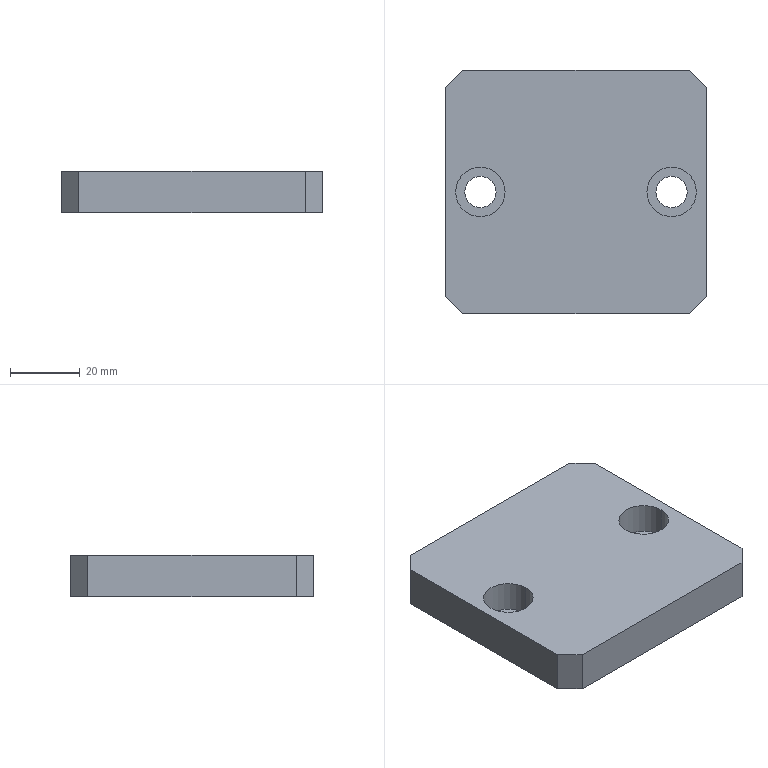Part | Creo | 1 solid | 20 faces | box 75 x 70 x 12 mm | volume 59148 mm3 | plane 12 | cylinder 8 | commonest cylinder face diameters 9 x4 14.25 x4
STEP:
#1=CARTESIAN_POINT('',(0.,0.,0.));
#2=DIRECTION('',(0.,0.,1.));
#3=DIRECTION('',(1.,0.,0.));
#4=AXIS2_PLACEMENT_3D('',#1,#2,#3);
#5=CARTESIAN_POINT('',(311.601,202.373,-28.441));
#6=VERTEX_POINT('',#5);
#7=CARTESIAN_POINT('',(311.601,262.373,-28.441));
#8=VERTEX_POINT('',#7);
#9=CARTESIAN_POINT('',(311.601,202.373,-28.441));
#10=DIRECTION('',(0.,1.,0.));
#11=VECTOR('',#10,60.);
#12=LINE('',#9,#11);
#13=EDGE_CURVE('',#6,#8,#12,.T.);
#14=ORIENTED_EDGE('',*,*,#13,.T.);
#15=CARTESIAN_POINT('',(316.601,267.373,-28.441));
#16=VERTEX_POINT('',#15);
#17=CARTESIAN_POINT('',(316.601,267.373,-28.441));
#18=DIRECTION('',(-0.7071,-0.7071,0.));
#19=VECTOR('',#18,7.071);
#20=LINE('',#17,#19);
#21=EDGE_CURVE('',#16,#8,#20,.T.);
#22=ORIENTED_EDGE('',*,*,#21,.F.);
#23=CARTESIAN_POINT('',(381.601,267.373,-28.441));
#24=VERTEX_POINT('',#23);
#25=CARTESIAN_POINT('',(316.601,267.373,-28.441));
#26=DIRECTION('',(1.,0.,0.));
#27=VECTOR('',#26,65.);
#28=LINE('',#25,#27);
#29=EDGE_CURVE('',#16,#24,#28,.T.);
#30=ORIENTED_EDGE('',*,*,#29,.T.);
#31=CARTESIAN_POINT('',(386.601,262.373,-28.441));
#32=VERTEX_POINT('',#31);
#33=CARTESIAN_POINT('',(386.601,262.373,-28.441));
#34=DIRECTION('',(-0.7071,0.7071,0.));
#35=VECTOR('',#34,7.071);
#36=LINE('',#33,#35);
#37=EDGE_CURVE('',#32,#24,#36,.T.);
#38=ORIENTED_EDGE('',*,*,#37,.F.);
#39=CARTESIAN_POINT('',(386.601,202.373,-28.441));
#40=VERTEX_POINT('',#39);
#41=CARTESIAN_POINT('',(386.601,262.373,-28.441));
#42=DIRECTION('',(0.,-1.,0.));
#43=VECTOR('',#42,60.);
#44=LINE('',#41,#43);
#45=EDGE_CURVE('',#32,#40,#44,.T.);
#46=ORIENTED_EDGE('',*,*,#45,.T.);
#47=CARTESIAN_POINT('',(381.601,197.373,-28.441));
#48=VERTEX_POINT('',#47);
#49=CARTESIAN_POINT('',(381.601,197.373,-28.441));
#50=DIRECTION('',(0.7071,0.7071,0.));
#51=VECTOR('',#50,7.071);
#52=LINE('',#49,#51);
#53=EDGE_CURVE('',#48,#40,#52,.T.);
#54=ORIENTED_EDGE('',*,*,#53,.F.);
#55=CARTESIAN_POINT('',(316.601,197.373,-28.441));
#56=VERTEX_POINT('',#55);
#57=CARTESIAN_POINT('',(381.601,197.373,-28.441));
#58=DIRECTION('',(-1.,0.,0.));
#59=VECTOR('',#58,65.);
#60=LINE('',#57,#59);
#61=EDGE_CURVE('',#48,#56,#60,.T.);
#62=ORIENTED_EDGE('',*,*,#61,.T.);
#63=CARTESIAN_POINT('',(311.601,202.373,-28.441));
#64=DIRECTION('',(0.7071,-0.7071,0.));
#65=VECTOR('',#64,7.071);
#66=LINE('',#63,#65);
#67=EDGE_CURVE('',#6,#56,#66,.T.);
#68=ORIENTED_EDGE('',*,*,#67,.F.);
#69=EDGE_LOOP('',(#14,#22,#30,#38,#46,#54,#62,#68));
#70=FACE_OUTER_BOUND('',#69,.F.);
#71=CARTESIAN_POINT('',(369.476,232.373,-28.441));
#72=VERTEX_POINT('',#71);
#73=CARTESIAN_POINT('',(383.726,232.373,-28.441));
#74=VERTEX_POINT('',#73);
#75=CARTESIAN_POINT('',(376.601,232.373,-28.441));
#76=DIRECTION('',(0.,0.,-1.));
#77=DIRECTION('',(-1.,0.,0.));
#78=AXIS2_PLACEMENT_3D('',#75,#76,#77);
#79=CIRCLE('',#78,7.125);
#80=EDGE_CURVE('',#72,#74,#79,.T.);
#81=ORIENTED_EDGE('',*,*,#80,.F.);
#82=CARTESIAN_POINT('',(376.601,232.373,-28.441));
#83=DIRECTION('',(0.,0.,-1.));
#84=DIRECTION('',(1.,0.,0.));
#85=AXIS2_PLACEMENT_3D('',#82,#83,#84);
#86=CIRCLE('',#85,7.125);
#87=EDGE_CURVE('',#74,#72,#86,.T.);
#88=ORIENTED_EDGE('',*,*,#87,.F.);
#89=EDGE_LOOP('',(#81,#88));
#90=FACE_BOUND('',#89,.F.);
#91=CARTESIAN_POINT('',(314.476,232.373,-28.441));
#92=VERTEX_POINT('',#91);
#93=CARTESIAN_POINT('',(328.726,232.373,-28.441));
#94=VERTEX_POINT('',#93);
#95=CARTESIAN_POINT('',(321.601,232.373,-28.441));
#96=DIRECTION('',(0.,0.,-1.));
#97=DIRECTION('',(-1.,0.,0.));
#98=AXIS2_PLACEMENT_3D('',#95,#96,#97);
#99=CIRCLE('',#98,7.125);
#100=EDGE_CURVE('',#92,#94,#99,.T.);
#101=ORIENTED_EDGE('',*,*,#100,.F.);
#102=CARTESIAN_POINT('',(321.601,232.373,-28.441));
#103=DIRECTION('',(0.,0.,-1.));
#104=DIRECTION('',(1.,0.,0.));
#105=AXIS2_PLACEMENT_3D('',#102,#103,#104);
#106=CIRCLE('',#105,7.125);
#107=EDGE_CURVE('',#94,#92,#106,.T.);
#108=ORIENTED_EDGE('',*,*,#107,.F.);
#109=EDGE_LOOP('',(#101,#108));
#110=FACE_BOUND('',#109,.F.);
#111=CARTESIAN_POINT('',(286.601,197.373,-28.441));
#112=DIRECTION('',(0.,0.,-1.));
#113=DIRECTION('',(-1.,0.,0.));
#114=AXIS2_PLACEMENT_3D('',#111,#112,#113);
#115=PLANE('',#114);
#116=ADVANCED_FACE('',(#70,#90,#110),#115,.F.);
#117=ORIENTED_EDGE('',*,*,#80,.T.);
#118=CARTESIAN_POINT('',(383.726,232.373,-37.441));
#119=VERTEX_POINT('',#118);
#120=CARTESIAN_POINT('',(383.726,232.373,-37.441));
#121=DIRECTION('',(0.,0.,1.));
#122=VECTOR('',#121,9.);
#123=LINE('',#120,#122);
#124=EDGE_CURVE('',#119,#74,#123,.T.);
#125=ORIENTED_EDGE('',*,*,#124,.F.);
#126=CARTESIAN_POINT('',(369.476,232.373,-37.441));
#127=VERTEX_POINT('',#126);
#128=CARTESIAN_POINT('',(376.601,232.373,-37.441));
#129=DIRECTION('',(0.,0.,1.));
#130=DIRECTION('',(1.,0.,0.));
#131=AXIS2_PLACEMENT_3D('',#128,#129,#130);
#132=CIRCLE('',#131,7.125);
#133=EDGE_CURVE('',#119,#127,#132,.T.);
#134=ORIENTED_EDGE('',*,*,#133,.T.);
#135=CARTESIAN_POINT('',(369.476,232.373,-37.441));
#136=DIRECTION('',(0.,0.,1.));
#137=VECTOR('',#136,9.);
#138=LINE('',#135,#137);
#139=EDGE_CURVE('',#127,#72,#138,.T.);
#140=ORIENTED_EDGE('',*,*,#139,.T.);
#141=EDGE_LOOP('',(#117,#125,#134,#140));
#142=FACE_OUTER_BOUND('',#141,.F.);
#143=CARTESIAN_POINT('',(376.601,232.373,-37.441));
#144=DIRECTION('',(0.,0.,1.));
#145=DIRECTION('',(1.,0.,0.));
#146=AXIS2_PLACEMENT_3D('',#143,#144,#145);
#147=CYLINDRICAL_SURFACE('',#146,7.125);
#148=ADVANCED_FACE('',(#142),#147,.F.);
#149=ORIENTED_EDGE('',*,*,#87,.T.);
#150=ORIENTED_EDGE('',*,*,#139,.F.);
#151=CARTESIAN_POINT('',(376.601,232.373,-37.441));
#152=DIRECTION('',(0.,0.,1.));
#153=DIRECTION('',(-1.,0.,0.));
#154=AXIS2_PLACEMENT_3D('',#151,#152,#153);
#155=CIRCLE('',#154,7.125);
#156=EDGE_CURVE('',#127,#119,#155,.T.);
#157=ORIENTED_EDGE('',*,*,#156,.T.);
#158=ORIENTED_EDGE('',*,*,#124,.T.);
#159=EDGE_LOOP('',(#149,#150,#157,#158));
#160=FACE_OUTER_BOUND('',#159,.F.);
#161=CARTESIAN_POINT('',(376.601,232.373,-37.441));
#162=DIRECTION('',(0.,0.,1.));
#163=DIRECTION('',(1.,0.,0.));
#164=AXIS2_PLACEMENT_3D('',#161,#162,#163);
#165=CYLINDRICAL_SURFACE('',#164,7.125);
#166=ADVANCED_FACE('',(#160),#165,.F.);
#167=ORIENTED_EDGE('',*,*,#156,.F.);
#168=ORIENTED_EDGE('',*,*,#133,.F.);
#169=EDGE_LOOP('',(#167,#168));
#170=FACE_OUTER_BOUND('',#169,.F.);
#171=CARTESIAN_POINT('',(381.101,232.373,-37.441));
#172=VERTEX_POINT('',#171);
#173=CARTESIAN_POINT('',(372.101,232.373,-37.441));
#174=VERTEX_POINT('',#173);
#175=CARTESIAN_POINT('',(376.601,232.373,-37.441));
#176=DIRECTION('',(0.,0.,-1.));
#177=DIRECTION('',(1.,0.,0.));
#178=AXIS2_PLACEMENT_3D('',#175,#176,#177);
#179=CIRCLE('',#178,4.5);
#180=EDGE_CURVE('',#172,#174,#179,.T.);
#181=ORIENTED_EDGE('',*,*,#180,.F.);
#182=CARTESIAN_POINT('',(376.601,232.373,-37.441));
#183=DIRECTION('',(0.,0.,-1.));
#184=DIRECTION('',(-1.,0.,0.));
#185=AXIS2_PLACEMENT_3D('',#182,#183,#184);
#186=CIRCLE('',#185,4.5);
#187=EDGE_CURVE('',#174,#172,#186,.T.);
#188=ORIENTED_EDGE('',*,*,#187,.F.);
#189=EDGE_LOOP('',(#181,#188));
#190=FACE_BOUND('',#189,.F.);
#191=CARTESIAN_POINT('',(376.601,232.373,-37.441));
#192=DIRECTION('',(0.,0.,-1.));
#193=DIRECTION('',(-1.,0.,0.));
#194=AXIS2_PLACEMENT_3D('',#191,#192,#193);
#195=PLANE('',#194);
#196=ADVANCED_FACE('',(#170,#190),#195,.F.);
#197=CARTESIAN_POINT('',(372.101,232.373,-40.441));
#198=VERTEX_POINT('',#197);
#199=CARTESIAN_POINT('',(381.101,232.373,-40.441));
#200=VERTEX_POINT('',#199);
#201=CARTESIAN_POINT('',(376.601,232.373,-40.441));
#202=DIRECTION('',(0.,0.,1.));
#203=DIRECTION('',(-1.,0.,0.));
#204=AXIS2_PLACEMENT_3D('',#201,#202,#203);
#205=CIRCLE('',#204,4.5);
#206=EDGE_CURVE('',#198,#200,#205,.T.);
#207=ORIENTED_EDGE('',*,*,#206,.T.);
#208=CARTESIAN_POINT('',(381.101,232.373,-37.441));
#209=DIRECTION('',(0.,0.,-1.));
#210=VECTOR('',#209,3.);
#211=LINE('',#208,#210);
#212=EDGE_CURVE('',#172,#200,#211,.T.);
#213=ORIENTED_EDGE('',*,*,#212,.F.);
#214=ORIENTED_EDGE('',*,*,#180,.T.);
#215=CARTESIAN_POINT('',(372.101,232.373,-37.441));
#216=DIRECTION('',(0.,0.,-1.));
#217=VECTOR('',#216,3.);
#218=LINE('',#215,#217);
#219=EDGE_CURVE('',#174,#198,#218,.T.);
#220=ORIENTED_EDGE('',*,*,#219,.T.);
#221=EDGE_LOOP('',(#207,#213,#214,#220));
#222=FACE_OUTER_BOUND('',#221,.F.);
#223=CARTESIAN_POINT('',(376.601,232.373,-37.441));
#224=DIRECTION('',(0.,0.,-1.));
#225=DIRECTION('',(-1.,0.,0.));
#226=AXIS2_PLACEMENT_3D('',#223,#224,#225);
#227=CYLINDRICAL_SURFACE('',#226,4.5);
#228=ADVANCED_FACE('',(#222),#227,.F.);
#229=CARTESIAN_POINT('',(381.601,197.373,-40.441));
#230=VERTEX_POINT('',#229);
#231=CARTESIAN_POINT('',(316.601,197.373,-40.441));
#232=VERTEX_POINT('',#231);
#233=CARTESIAN_POINT('',(381.601,197.373,-40.441));
#234=DIRECTION('',(-1.,0.,0.));
#235=VECTOR('',#234,65.);
#236=LINE('',#233,#235);
#237=EDGE_CURVE('',#230,#232,#236,.T.);
#238=ORIENTED_EDGE('',*,*,#237,.F.);
#239=CARTESIAN_POINT('',(386.601,202.373,-40.441));
#240=VERTEX_POINT('',#239);
#241=CARTESIAN_POINT('',(386.601,202.373,-40.441));
#242=DIRECTION('',(-0.7071,-0.7071,0.));
#243=VECTOR('',#242,7.071);
#244=LINE('',#241,#243);
#245=EDGE_CURVE('',#240,#230,#244,.T.);
#246=ORIENTED_EDGE('',*,*,#245,.F.);
#247=CARTESIAN_POINT('',(386.601,262.373,-40.441));
#248=VERTEX_POINT('',#247);
#249=CARTESIAN_POINT('',(386.601,262.373,-40.441));
#250=DIRECTION('',(0.,-1.,0.));
#251=VECTOR('',#250,60.);
#252=LINE('',#249,#251);
#253=EDGE_CURVE('',#248,#240,#252,.T.);
#254=ORIENTED_EDGE('',*,*,#253,.F.);
#255=CARTESIAN_POINT('',(381.601,267.373,-40.441));
#256=VERTEX_POINT('',#255);
#257=CARTESIAN_POINT('',(381.601,267.373,-40.441));
#258=DIRECTION('',(0.7071,-0.7071,0.));
#259=VECTOR('',#258,7.071);
#260=LINE('',#257,#259);
#261=EDGE_CURVE('',#256,#248,#260,.T.);
#262=ORIENTED_EDGE('',*,*,#261,.F.);
#263=CARTESIAN_POINT('',(316.601,267.373,-40.441));
#264=VERTEX_POINT('',#263);
#265=CARTESIAN_POINT('',(316.601,267.373,-40.441));
#266=DIRECTION('',(1.,0.,0.));
#267=VECTOR('',#266,65.);
#268=LINE('',#265,#267);
#269=EDGE_CURVE('',#264,#256,#268,.T.);
#270=ORIENTED_EDGE('',*,*,#269,.F.);
#271=CARTESIAN_POINT('',(311.601,262.373,-40.441));
#272=VERTEX_POINT('',#271);
#273=CARTESIAN_POINT('',(311.601,262.373,-40.441));
#274=DIRECTION('',(0.7071,0.7071,0.));
#275=VECTOR('',#274,7.071);
#276=LINE('',#273,#275);
#277=EDGE_CURVE('',#272,#264,#276,.T.);
#278=ORIENTED_EDGE('',*,*,#277,.F.);
#279=CARTESIAN_POINT('',(311.601,202.373,-40.441));
#280=VERTEX_POINT('',#279);
#281=CARTESIAN_POINT('',(311.601,202.373,-40.441));
#282=DIRECTION('',(0.,1.,0.));
#283=VECTOR('',#282,60.);
#284=LINE('',#281,#283);
#285=EDGE_CURVE('',#280,#272,#284,.T.);
#286=ORIENTED_EDGE('',*,*,#285,.F.);
#287=CARTESIAN_POINT('',(316.601,197.373,-40.441));
#288=DIRECTION('',(-0.7071,0.7071,0.));
#289=VECTOR('',#288,7.071);
#290=LINE('',#287,#289);
#291=EDGE_CURVE('',#232,#280,#290,.T.);
#292=ORIENTED_EDGE('',*,*,#291,.F.);
#293=EDGE_LOOP('',(#238,#246,#254,#262,#270,#278,#286,#292));
#294=FACE_OUTER_BOUND('',#293,.F.);
#295=ORIENTED_EDGE('',*,*,#206,.F.);
#296=CARTESIAN_POINT('',(376.601,232.373,-40.441));
#297=DIRECTION('',(0.,0.,1.));
#298=DIRECTION('',(1.,0.,0.));
#299=AXIS2_PLACEMENT_3D('',#296,#297,#298);
#300=CIRCLE('',#299,4.5);
#301=EDGE_CURVE('',#200,#198,#300,.T.);
#302=ORIENTED_EDGE('',*,*,#301,.F.);
#303=EDGE_LOOP('',(#295,#302));
#304=FACE_BOUND('',#303,.F.);
#305=CARTESIAN_POINT('',(317.101,232.373,-40.441));
#306=VERTEX_POINT('',#305);
#307=CARTESIAN_POINT('',(326.101,232.373,-40.441));
#308=VERTEX_POINT('',#307);
#309=CARTESIAN_POINT('',(321.601,232.373,-40.441));
#310=DIRECTION('',(0.,0.,1.));
#311=DIRECTION('',(-1.,0.,0.));
#312=AXIS2_PLACEMENT_3D('',#309,#310,#311);
#313=CIRCLE('',#312,4.5);
#314=EDGE_CURVE('',#306,#308,#313,.T.);
#315=ORIENTED_EDGE('',*,*,#314,.F.);
#316=CARTESIAN_POINT('',(321.601,232.373,-40.441));
#317=DIRECTION('',(0.,0.,1.));
#318=DIRECTION('',(1.,0.,0.));
#319=AXIS2_PLACEMENT_3D('',#316,#317,#318);
#320=CIRCLE('',#319,4.5);
#321=EDGE_CURVE('',#308,#306,#320,.T.);
#322=ORIENTED_EDGE('',*,*,#321,.F.);
#323=EDGE_LOOP('',(#315,#322));
#324=FACE_BOUND('',#323,.F.);
#325=CARTESIAN_POINT('',(286.601,197.373,-40.441));
#326=DIRECTION('',(0.,0.,-1.));
#327=DIRECTION('',(-1.,0.,0.));
#328=AXIS2_PLACEMENT_3D('',#325,#326,#327);
#329=PLANE('',#328);
#330=ADVANCED_FACE('',(#294,#304,#324),#329,.T.);
#331=ORIENTED_EDGE('',*,*,#314,.T.);
#332=CARTESIAN_POINT('',(326.101,232.373,-37.441));
#333=VERTEX_POINT('',#332);
#334=CARTESIAN_POINT('',(326.101,232.373,-37.441));
#335=DIRECTION('',(0.,0.,-1.));
#336=VECTOR('',#335,3.);
#337=LINE('',#334,#336);
#338=EDGE_CURVE('',#333,#308,#337,.T.);
#339=ORIENTED_EDGE('',*,*,#338,.F.);
#340=CARTESIAN_POINT('',(317.101,232.373,-37.441));
#341=VERTEX_POINT('',#340);
#342=CARTESIAN_POINT('',(321.601,232.373,-37.441));
#343=DIRECTION('',(0.,0.,-1.));
#344=DIRECTION('',(1.,0.,0.));
#345=AXIS2_PLACEMENT_3D('',#342,#343,#344);
#346=CIRCLE('',#345,4.5);
#347=EDGE_CURVE('',#333,#341,#346,.T.);
#348=ORIENTED_EDGE('',*,*,#347,.T.);
#349=CARTESIAN_POINT('',(317.101,232.373,-37.441));
#350=DIRECTION('',(0.,0.,-1.));
#351=VECTOR('',#350,3.);
#352=LINE('',#349,#351);
#353=EDGE_CURVE('',#341,#306,#352,.T.);
#354=ORIENTED_EDGE('',*,*,#353,.T.);
#355=EDGE_LOOP('',(#331,#339,#348,#354));
#356=FACE_OUTER_BOUND('',#355,.F.);
#357=CARTESIAN_POINT('',(321.601,232.373,-37.441));
#358=DIRECTION('',(0.,0.,-1.));
#359=DIRECTION('',(-1.,0.,0.));
#360=AXIS2_PLACEMENT_3D('',#357,#358,#359);
#361=CYLINDRICAL_SURFACE('',#360,4.5);
#362=ADVANCED_FACE('',(#356),#361,.F.);
#363=ORIENTED_EDGE('',*,*,#321,.T.);
#364=ORIENTED_EDGE('',*,*,#353,.F.);
#365=CARTESIAN_POINT('',(321.601,232.373,-37.441));
#366=DIRECTION('',(0.,0.,-1.));
#367=DIRECTION('',(-1.,0.,0.));
#368=AXIS2_PLACEMENT_3D('',#365,#366,#367);
#369=CIRCLE('',#368,4.5);
#370=EDGE_CURVE('',#341,#333,#369,.T.);
#371=ORIENTED_EDGE('',*,*,#370,.T.);
#372=ORIENTED_EDGE('',*,*,#338,.T.);
#373=EDGE_LOOP('',(#363,#364,#371,#372));
#374=FACE_OUTER_BOUND('',#373,.F.);
#375=CARTESIAN_POINT('',(321.601,232.373,-37.441));
#376=DIRECTION('',(0.,0.,-1.));
#377=DIRECTION('',(-1.,0.,0.));
#378=AXIS2_PLACEMENT_3D('',#375,#376,#377);
#379=CYLINDRICAL_SURFACE('',#378,4.5);
#380=ADVANCED_FACE('',(#374),#379,.F.);
#381=CARTESIAN_POINT('',(314.476,232.373,-37.441));
#382=VERTEX_POINT('',#381);
#383=CARTESIAN_POINT('',(328.726,232.373,-37.441));
#384=VERTEX_POINT('',#383);
#385=CARTESIAN_POINT('',(321.601,232.373,-37.441));
#386=DIRECTION('',(0.,0.,1.));
#387=DIRECTION('',(-1.,0.,0.));
#388=AXIS2_PLACEMENT_3D('',#385,#386,#387);
#389=CIRCLE('',#388,7.125);
#390=EDGE_CURVE('',#382,#384,#389,.T.);
#391=ORIENTED_EDGE('',*,*,#390,.F.);
#392=CARTESIAN_POINT('',(321.601,232.373,-37.441));
#393=DIRECTION('',(0.,0.,1.));
#394=DIRECTION('',(1.,0.,0.));
#395=AXIS2_PLACEMENT_3D('',#392,#393,#394);
#396=CIRCLE('',#395,7.125);
#397=EDGE_CURVE('',#384,#382,#396,.T.);
#398=ORIENTED_EDGE('',*,*,#397,.F.);
#399=EDGE_LOOP('',(#391,#398));
#400=FACE_OUTER_BOUND('',#399,.F.);
#401=ORIENTED_EDGE('',*,*,#347,.F.);
#402=ORIENTED_EDGE('',*,*,#370,.F.);
#403=EDGE_LOOP('',(#401,#402));
#404=FACE_BOUND('',#403,.F.);
#405=CARTESIAN_POINT('',(321.601,232.373,-37.441));
#406=DIRECTION('',(0.,0.,-1.));
#407=DIRECTION('',(-1.,0.,0.));
#408=AXIS2_PLACEMENT_3D('',#405,#406,#407);
#409=PLANE('',#408);
#410=ADVANCED_FACE('',(#400,#404),#409,.F.);
#411=ORIENTED_EDGE('',*,*,#107,.T.);
#412=CARTESIAN_POINT('',(314.476,232.373,-37.441));
#413=DIRECTION('',(0.,0.,1.));
#414=VECTOR('',#413,9.);
#415=LINE('',#412,#414);
#416=EDGE_CURVE('',#382,#92,#415,.T.);
#417=ORIENTED_EDGE('',*,*,#416,.F.);
#418=ORIENTED_EDGE('',*,*,#390,.T.);
#419=CARTESIAN_POINT('',(328.726,232.373,-37.441));
#420=DIRECTION('',(0.,0.,1.));
#421=VECTOR('',#420,9.);
#422=LINE('',#419,#421);
#423=EDGE_CURVE('',#384,#94,#422,.T.);
#424=ORIENTED_EDGE('',*,*,#423,.T.);
#425=EDGE_LOOP('',(#411,#417,#418,#424));
#426=FACE_OUTER_BOUND('',#425,.F.);
#427=CARTESIAN_POINT('',(321.601,232.373,-37.441));
#428=DIRECTION('',(0.,0.,1.));
#429=DIRECTION('',(1.,0.,0.));
#430=AXIS2_PLACEMENT_3D('',#427,#428,#429);
#431=CYLINDRICAL_SURFACE('',#430,7.125);
#432=ADVANCED_FACE('',(#426),#431,.F.);
#433=ORIENTED_EDGE('',*,*,#100,.T.);
#434=ORIENTED_EDGE('',*,*,#423,.F.);
#435=ORIENTED_EDGE('',*,*,#397,.T.);
#436=ORIENTED_EDGE('',*,*,#416,.T.);
#437=EDGE_LOOP('',(#433,#434,#435,#436));
#438=FACE_OUTER_BOUND('',#437,.F.);
#439=CARTESIAN_POINT('',(321.601,232.373,-37.441));
#440=DIRECTION('',(0.,0.,1.));
#441=DIRECTION('',(1.,0.,0.));
#442=AXIS2_PLACEMENT_3D('',#439,#440,#441);
#443=CYLINDRICAL_SURFACE('',#442,7.125);
#444=ADVANCED_FACE('',(#438),#443,.F.);
#445=ORIENTED_EDGE('',*,*,#301,.T.);
#446=ORIENTED_EDGE('',*,*,#219,.F.);
#447=ORIENTED_EDGE('',*,*,#187,.T.);
#448=ORIENTED_EDGE('',*,*,#212,.T.);
#449=EDGE_LOOP('',(#445,#446,#447,#448));
#450=FACE_OUTER_BOUND('',#449,.F.);
#451=CARTESIAN_POINT('',(376.601,232.373,-37.441));
#452=DIRECTION('',(0.,0.,-1.));
#453=DIRECTION('',(-1.,0.,0.));
#454=AXIS2_PLACEMENT_3D('',#451,#452,#453);
#455=CYLINDRICAL_SURFACE('',#454,4.5);
#456=ADVANCED_FACE('',(#450),#455,.F.);
#457=ORIENTED_EDGE('',*,*,#61,.F.);
#458=CARTESIAN_POINT('',(381.601,197.373,-28.441));
#459=DIRECTION('',(0.,0.,-1.));
#460=VECTOR('',#459,12.);
#461=LINE('',#458,#460);
#462=EDGE_CURVE('',#48,#230,#461,.T.);
#463=ORIENTED_EDGE('',*,*,#462,.T.);
#464=ORIENTED_EDGE('',*,*,#237,.T.);
#465=CARTESIAN_POINT('',(316.601,197.373,-40.441));
#466=DIRECTION('',(0.,0.,1.));
#467=VECTOR('',#466,12.);
#468=LINE('',#465,#467);
#469=EDGE_CURVE('',#232,#56,#468,.T.);
#470=ORIENTED_EDGE('',*,*,#469,.T.);
#471=EDGE_LOOP('',(#457,#463,#464,#470));
#472=FACE_OUTER_BOUND('',#471,.F.);
#473=CARTESIAN_POINT('',(286.601,197.373,-40.441));
#474=DIRECTION('',(0.,1.,0.));
#475=DIRECTION('',(0.,0.,1.));
#476=AXIS2_PLACEMENT_3D('',#473,#474,#475);
#477=PLANE('',#476);
#478=ADVANCED_FACE('',(#472),#477,.F.);
#479=ORIENTED_EDGE('',*,*,#245,.T.);
#480=ORIENTED_EDGE('',*,*,#462,.F.);
#481=ORIENTED_EDGE('',*,*,#53,.T.);
#482=CARTESIAN_POINT('',(386.601,202.373,-40.441));
#483=DIRECTION('',(0.,0.,1.));
#484=VECTOR('',#483,12.);
#485=LINE('',#482,#484);
#486=EDGE_CURVE('',#240,#40,#485,.T.);
#487=ORIENTED_EDGE('',*,*,#486,.F.);
#488=EDGE_LOOP('',(#479,#480,#481,#487));
#489=FACE_OUTER_BOUND('',#488,.F.);
#490=CARTESIAN_POINT('',(381.601,197.373,-40.441));
#491=DIRECTION('',(-0.7071,0.7071,0.));
#492=DIRECTION('',(-0.7071,-0.7071,0.));
#493=AXIS2_PLACEMENT_3D('',#490,#491,#492);
#494=PLANE('',#493);
#495=ADVANCED_FACE('',(#489),#494,.F.);
#496=ORIENTED_EDGE('',*,*,#45,.F.);
#497=CARTESIAN_POINT('',(386.601,262.373,-28.441));
#498=DIRECTION('',(0.,0.,-1.));
#499=VECTOR('',#498,12.);
#500=LINE('',#497,#499);
#501=EDGE_CURVE('',#32,#248,#500,.T.);
#502=ORIENTED_EDGE('',*,*,#501,.T.);
#503=ORIENTED_EDGE('',*,*,#253,.T.);
#504=ORIENTED_EDGE('',*,*,#486,.T.);
#505=EDGE_LOOP('',(#496,#502,#503,#504));
#506=FACE_OUTER_BOUND('',#505,.F.);
#507=CARTESIAN_POINT('',(386.601,197.373,-40.441));
#508=DIRECTION('',(-1.,0.,0.));
#509=DIRECTION('',(0.,0.,1.));
#510=AXIS2_PLACEMENT_3D('',#507,#508,#509);
#511=PLANE('',#510);
#512=ADVANCED_FACE('',(#506),#511,.F.);
#513=ORIENTED_EDGE('',*,*,#261,.T.);
#514=ORIENTED_EDGE('',*,*,#501,.F.);
#515=ORIENTED_EDGE('',*,*,#37,.T.);
#516=CARTESIAN_POINT('',(381.601,267.373,-40.441));
#517=DIRECTION('',(0.,0.,1.));
#518=VECTOR('',#517,12.);
#519=LINE('',#516,#518);
#520=EDGE_CURVE('',#256,#24,#519,.T.);
#521=ORIENTED_EDGE('',*,*,#520,.F.);
#522=EDGE_LOOP('',(#513,#514,#515,#521));
#523=FACE_OUTER_BOUND('',#522,.F.);
#524=CARTESIAN_POINT('',(386.601,262.373,-40.441));
#525=DIRECTION('',(-0.7071,-0.7071,0.));
#526=DIRECTION('',(0.7071,-0.7071,0.));
#527=AXIS2_PLACEMENT_3D('',#524,#525,#526);
#528=PLANE('',#527);
#529=ADVANCED_FACE('',(#523),#528,.F.);
#530=ORIENTED_EDGE('',*,*,#269,.T.);
#531=ORIENTED_EDGE('',*,*,#520,.T.);
#532=ORIENTED_EDGE('',*,*,#29,.F.);
#533=CARTESIAN_POINT('',(316.601,267.373,-28.441));
#534=DIRECTION('',(0.,0.,-1.));
#535=VECTOR('',#534,12.);
#536=LINE('',#533,#535);
#537=EDGE_CURVE('',#16,#264,#536,.T.);
#538=ORIENTED_EDGE('',*,*,#537,.T.);
#539=EDGE_LOOP('',(#530,#531,#532,#538));
#540=FACE_OUTER_BOUND('',#539,.F.);
#541=CARTESIAN_POINT('',(386.601,267.373,-40.441));
#542=DIRECTION('',(0.,-1.,0.));
#543=DIRECTION('',(0.,0.,-1.));
#544=AXIS2_PLACEMENT_3D('',#541,#542,#543);
#545=PLANE('',#544);
#546=ADVANCED_FACE('',(#540),#545,.F.);
#547=ORIENTED_EDGE('',*,*,#277,.T.);
#548=ORIENTED_EDGE('',*,*,#537,.F.);
#549=ORIENTED_EDGE('',*,*,#21,.T.);
#550=CARTESIAN_POINT('',(311.601,262.373,-40.441));
#551=DIRECTION('',(0.,0.,1.));
#552=VECTOR('',#551,12.);
#553=LINE('',#550,#552);
#554=EDGE_CURVE('',#272,#8,#553,.T.);
#555=ORIENTED_EDGE('',*,*,#554,.F.);
#556=EDGE_LOOP('',(#547,#548,#549,#555));
#557=FACE_OUTER_BOUND('',#556,.F.);
#558=CARTESIAN_POINT('',(316.601,267.373,-40.441));
#559=DIRECTION('',(0.7071,-0.7071,0.));
#560=DIRECTION('',(0.7071,0.7071,0.));
#561=AXIS2_PLACEMENT_3D('',#558,#559,#560);
#562=PLANE('',#561);
#563=ADVANCED_FACE('',(#557),#562,.F.);
#564=ORIENTED_EDGE('',*,*,#285,.T.);
#565=ORIENTED_EDGE('',*,*,#554,.T.);
#566=ORIENTED_EDGE('',*,*,#13,.F.);
#567=CARTESIAN_POINT('',(311.601,202.373,-28.441));
#568=DIRECTION('',(0.,0.,-1.));
#569=VECTOR('',#568,12.);
#570=LINE('',#567,#569);
#571=EDGE_CURVE('',#6,#280,#570,.T.);
#572=ORIENTED_EDGE('',*,*,#571,.T.);
#573=EDGE_LOOP('',(#564,#565,#566,#572));
#574=FACE_OUTER_BOUND('',#573,.F.);
#575=CARTESIAN_POINT('',(311.601,267.373,-40.441));
#576=DIRECTION('',(1.,0.,0.));
#577=DIRECTION('',(0.,0.,-1.));
#578=AXIS2_PLACEMENT_3D('',#575,#576,#577);
#579=PLANE('',#578);
#580=ADVANCED_FACE('',(#574),#579,.F.);
#581=ORIENTED_EDGE('',*,*,#291,.T.);
#582=ORIENTED_EDGE('',*,*,#571,.F.);
#583=ORIENTED_EDGE('',*,*,#67,.T.);
#584=ORIENTED_EDGE('',*,*,#469,.F.);
#585=EDGE_LOOP('',(#581,#582,#583,#584));
#586=FACE_OUTER_BOUND('',#585,.F.);
#587=CARTESIAN_POINT('',(311.601,202.373,-40.441));
#588=DIRECTION('',(0.7071,0.7071,0.));
#589=DIRECTION('',(-0.7071,0.7071,0.));
#590=AXIS2_PLACEMENT_3D('',#587,#588,#589);
#591=PLANE('',#590);
#592=ADVANCED_FACE('',(#586),#591,.F.);
#593=CLOSED_SHELL('',(#116,#148,#166,#196,#228,#330,#362,#380,#410,#432,#444,#456,#478,#495,#512,#529,#546,#563,#580,#592));
#594=MANIFOLD_SOLID_BREP('',#593);
#595=(LENGTH_UNIT()NAMED_UNIT(*)SI_UNIT(.MILLI.,.METRE.));
#596=UNCERTAINTY_MEASURE_WITH_UNIT(LENGTH_MEASURE(0.01033),#595,'','');
#597=(NAMED_UNIT(*)PLANE_ANGLE_UNIT()SI_UNIT($,.RADIAN.));
#598=PLANE_ANGLE_MEASURE_WITH_UNIT(PLANE_ANGLE_MEASURE(0.01745),#597);
#599=(CONVERSION_BASED_UNIT('DEGREE',#598)NAMED_UNIT(*)PLANE_ANGLE_UNIT());
#600=(NAMED_UNIT(*)SI_UNIT($,.STERADIAN.)SOLID_ANGLE_UNIT());
#601=(GEOMETRIC_REPRESENTATION_CONTEXT(3)GLOBAL_UNCERTAINTY_ASSIGNED_CONTEXT((#596))GLOBAL_UNIT_ASSIGNED_CONTEXT((#595,#599,#600))REPRESENTATION_CONTEXT('',''));
#602=ADVANCED_BREP_SHAPE_REPRESENTATION('',(#4,#594),#601);